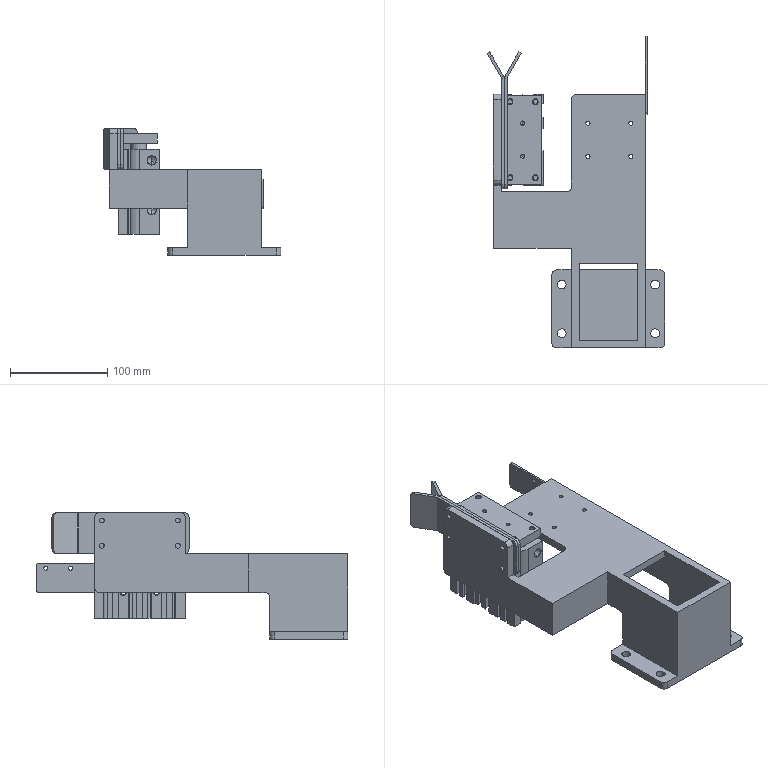Part | SolidWorks | features CompositeCurve 6 | 6 solids | 409 faces | box 182.598 x 320 x 130 mm | volume 852374 mm3 | plane 185 | cylinder 148 | cone 76 | commonest cylinder face diameters 4.917 x24 4 x22 10 x20 4.2 x12 5 x8 5.4 x8